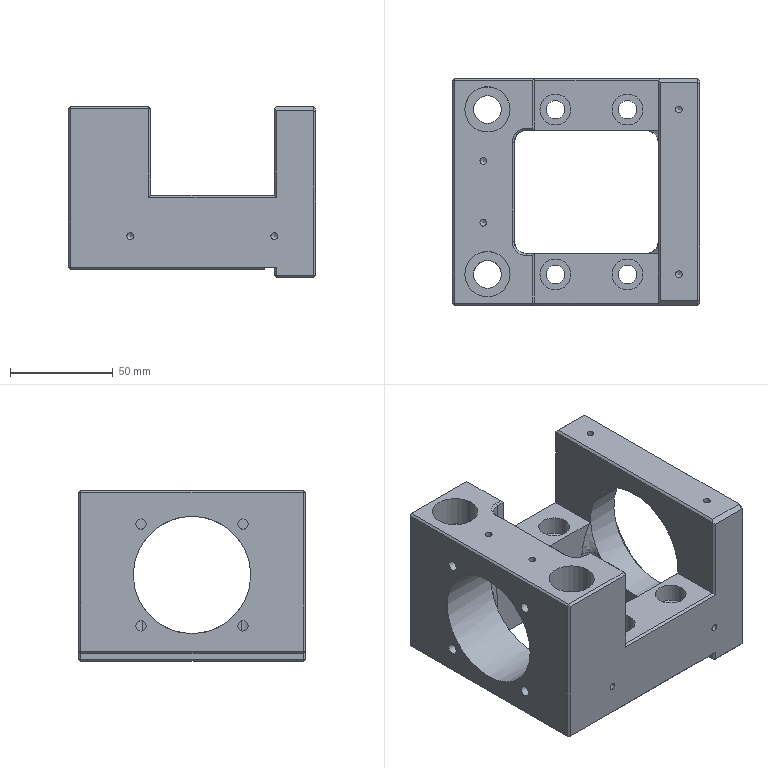Part | NX | 1 solid | 125 faces | box 120 x 110 x 83 mm | volume 406919 mm3 | plane 70 | cylinder 37 | cone 14 | spline 4 | commonest cylinder face diameters 3.3 x8 12 x6 4.2 x4 5 x4 9 x4 15 x4